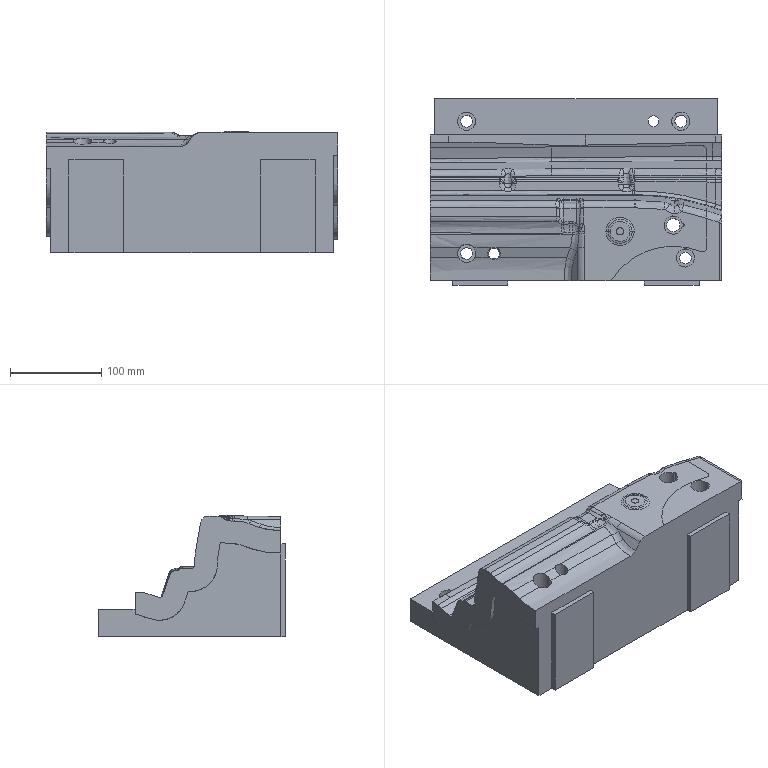Part | NX | features solid 2 | 1 solid | 254 faces | box 320.002 x 205 x 132.901 mm | volume 5227851 mm3 | spline 217 | plane 23 | cylinder 14 | commonest cylinder face diameters 20 x5 13 x4 12 x2 4 x1 14 x1 14.6 x1